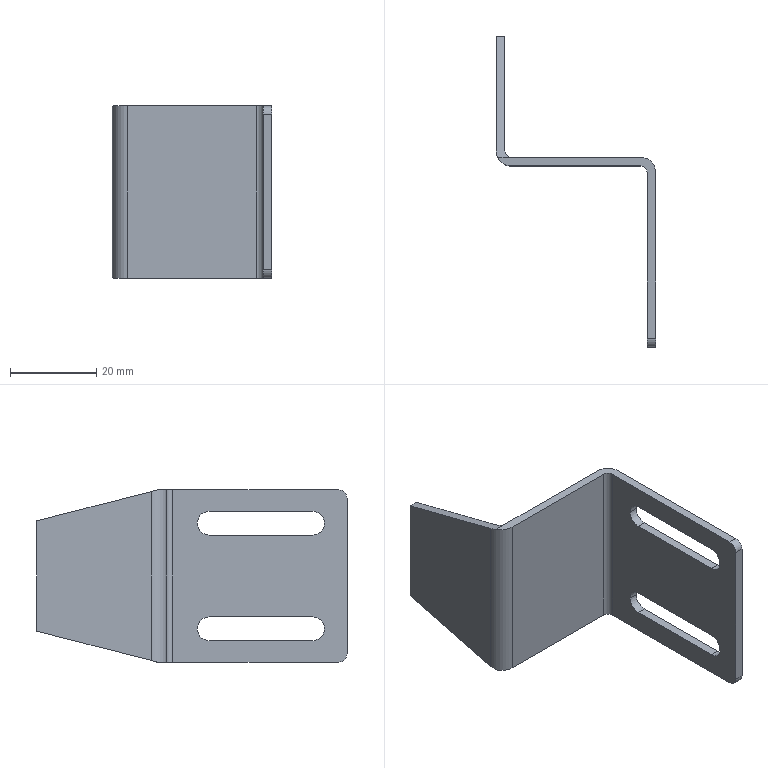Part | NX | features BREP 1 | 1 solid | 28 faces | box 37 x 72 x 40 mm | volume 7359 mm3 | plane 16 | cylinder 12 | commonest cylinder face diameters 5.5 x6 3 x2 4 x2 7 x2
STEP:
#1=CARTESIAN_POINT('',(0.,-7.25,-12.25));
#2=VERTEX_POINT('',#1);
#3=CARTESIAN_POINT('',(0.,-10.,-9.5));
#4=VERTEX_POINT('',#3);
#5=CARTESIAN_POINT('',(0.,-10.,-12.25));
#6=DIRECTION('',(1.,0.,0.));
#7=DIRECTION('',(0.,1.,0.));
#8=AXIS2_PLACEMENT_3D('',#5,#6,#7);
#9=CIRCLE('',#8,2.75);
#10=EDGE_CURVE('',#2,#4,#9,.T.);
#11=ORIENTED_EDGE('',*,*,#10,.F.);
#12=CARTESIAN_POINT('',(2.,-7.25,-12.25));
#13=VERTEX_POINT('',#12);
#14=CARTESIAN_POINT('',(-35.,-7.25,-12.25));
#15=DIRECTION('',(1.,0.,0.));
#16=VECTOR('',#15,1000.);
#17=LINE('',#14,#16);
#18=EDGE_CURVE('',#2,#13,#17,.T.);
#19=ORIENTED_EDGE('',*,*,#18,.T.);
#20=CARTESIAN_POINT('',(2.,-10.,-9.5));
#21=VERTEX_POINT('',#20);
#22=CARTESIAN_POINT('',(2.,-10.,-12.25));
#23=DIRECTION('',(1.,0.,0.));
#24=DIRECTION('',(0.,-1.,0.));
#25=AXIS2_PLACEMENT_3D('',#22,#23,#24);
#26=CIRCLE('',#25,2.75);
#27=EDGE_CURVE('',#13,#21,#26,.T.);
#28=ORIENTED_EDGE('',*,*,#27,.T.);
#29=CARTESIAN_POINT('',(-35.,-10.,-9.5));
#30=DIRECTION('',(1.,0.,0.));
#31=VECTOR('',#30,1000.);
#32=LINE('',#29,#31);
#33=EDGE_CURVE('',#4,#21,#32,.T.);
#34=ORIENTED_EDGE('',*,*,#33,.F.);
#35=EDGE_LOOP('',(#11,#19,#28,#34));
#36=FACE_BOUND('',#35,.T.);
#37=CARTESIAN_POINT('',(-35.,-10.,-12.25));
#38=DIRECTION('',(1.,0.,0.));
#39=DIRECTION('',(0.,1.,0.));
#40=AXIS2_PLACEMENT_3D('',#37,#38,#39);
#41=CYLINDRICAL_SURFACE('',#40,2.75);
#42=ADVANCED_FACE('',(#36),#41,.F.);
#43=CARTESIAN_POINT('',(0.,-7.25,12.25));
#44=VERTEX_POINT('',#43);
#45=CARTESIAN_POINT('',(0.,-10.,15.));
#46=VERTEX_POINT('',#45);
#47=CARTESIAN_POINT('',(0.,-10.,12.25));
#48=DIRECTION('',(1.,0.,0.));
#49=DIRECTION('',(0.,1.,0.));
#50=AXIS2_PLACEMENT_3D('',#47,#48,#49);
#51=CIRCLE('',#50,2.75);
#52=EDGE_CURVE('',#44,#46,#51,.T.);
#53=ORIENTED_EDGE('',*,*,#52,.F.);
#54=CARTESIAN_POINT('',(2.,-7.25,12.25));
#55=VERTEX_POINT('',#54);
#56=CARTESIAN_POINT('',(-35.,-7.25,12.25));
#57=DIRECTION('',(1.,0.,0.));
#58=VECTOR('',#57,1000.);
#59=LINE('',#56,#58);
#60=EDGE_CURVE('',#44,#55,#59,.T.);
#61=ORIENTED_EDGE('',*,*,#60,.T.);
#62=CARTESIAN_POINT('',(2.,-10.,15.));
#63=VERTEX_POINT('',#62);
#64=CARTESIAN_POINT('',(2.,-10.,12.25));
#65=DIRECTION('',(1.,0.,0.));
#66=DIRECTION('',(0.,1.,0.));
#67=AXIS2_PLACEMENT_3D('',#64,#65,#66);
#68=CIRCLE('',#67,2.75);
#69=EDGE_CURVE('',#55,#63,#68,.T.);
#70=ORIENTED_EDGE('',*,*,#69,.T.);
#71=CARTESIAN_POINT('',(-35.,-10.,15.));
#72=DIRECTION('',(1.,0.,0.));
#73=VECTOR('',#72,1000.);
#74=LINE('',#71,#73);
#75=EDGE_CURVE('',#46,#63,#74,.T.);
#76=ORIENTED_EDGE('',*,*,#75,.F.);
#77=EDGE_LOOP('',(#53,#61,#70,#76));
#78=FACE_BOUND('',#77,.T.);
#79=CARTESIAN_POINT('',(-35.,-10.,12.25));
#80=DIRECTION('',(1.,0.,0.));
#81=DIRECTION('',(0.,1.,0.));
#82=AXIS2_PLACEMENT_3D('',#79,#80,#81);
#83=CYLINDRICAL_SURFACE('',#82,2.75);
#84=ADVANCED_FACE('',(#78),#83,.F.);
#85=CARTESIAN_POINT('',(2.,-42.,18.));
#86=VERTEX_POINT('',#85);
#87=CARTESIAN_POINT('',(2.,-42.,-18.));
#88=VERTEX_POINT('',#87);
#89=CARTESIAN_POINT('',(2.,-42.,20.));
#90=DIRECTION('',(0.,0.,-1.));
#91=VECTOR('',#90,1000.);
#92=LINE('',#89,#91);
#93=EDGE_CURVE('',#86,#88,#92,.T.);
#94=ORIENTED_EDGE('',*,*,#93,.T.);
#95=CARTESIAN_POINT('',(2.,-40.,-20.));
#96=VERTEX_POINT('',#95);
#97=CARTESIAN_POINT('',(2.,-40.,-18.));
#98=DIRECTION('',(1.,0.,0.));
#99=DIRECTION('',(0.,-1.,0.));
#100=AXIS2_PLACEMENT_3D('',#97,#98,#99);
#101=CIRCLE('',#100,2.);
#102=EDGE_CURVE('',#88,#96,#101,.T.);
#103=ORIENTED_EDGE('',*,*,#102,.T.);
#104=CARTESIAN_POINT('',(2.,-1.5,-20.));
#105=VERTEX_POINT('',#104);
#106=CARTESIAN_POINT('',(2.,2.,-20.));
#107=DIRECTION('',(0.,1.,0.));
#108=VECTOR('',#107,1000.);
#109=LINE('',#106,#108);
#110=EDGE_CURVE('',#96,#105,#109,.T.);
#111=ORIENTED_EDGE('',*,*,#110,.T.);
#112=CARTESIAN_POINT('',(2.,-1.5,20.));
#113=VERTEX_POINT('',#112);
#114=CARTESIAN_POINT('',(2.,-1.5,20.));
#115=DIRECTION('',(0.,0.,1.));
#116=VECTOR('',#115,1000.);
#117=LINE('',#114,#116);
#118=EDGE_CURVE('',#105,#113,#117,.T.);
#119=ORIENTED_EDGE('',*,*,#118,.T.);
#120=CARTESIAN_POINT('',(2.,-40.,20.));
#121=VERTEX_POINT('',#120);
#122=CARTESIAN_POINT('',(2.,2.,20.));
#123=DIRECTION('',(0.,1.,0.));
#124=VECTOR('',#123,1000.);
#125=LINE('',#122,#124);
#126=EDGE_CURVE('',#121,#113,#125,.T.);
#127=ORIENTED_EDGE('',*,*,#126,.F.);
#128=CARTESIAN_POINT('',(2.,-40.,18.));
#129=DIRECTION('',(1.,0.,0.));
#130=DIRECTION('',(0.,-1.,0.));
#131=AXIS2_PLACEMENT_3D('',#128,#129,#130);
#132=CIRCLE('',#131,2.);
#133=EDGE_CURVE('',#121,#86,#132,.T.);
#134=ORIENTED_EDGE('',*,*,#133,.T.);
#135=EDGE_LOOP('',(#94,#103,#111,#119,#127,#134));
#136=FACE_BOUND('',#135,.T.);
#137=CARTESIAN_POINT('',(2.,-34.,-9.5));
#138=VERTEX_POINT('',#137);
#139=CARTESIAN_POINT('',(2.,-10.,-9.5));
#140=DIRECTION('',(0.,-1.,0.));
#141=VECTOR('',#140,1000.);
#142=LINE('',#139,#141);
#143=EDGE_CURVE('',#21,#138,#142,.T.);
#144=ORIENTED_EDGE('',*,*,#143,.F.);
#145=ORIENTED_EDGE('',*,*,#27,.F.);
#146=CARTESIAN_POINT('',(2.,-10.,-15.));
#147=VERTEX_POINT('',#146);
#148=CARTESIAN_POINT('',(2.,-10.,-12.25));
#149=DIRECTION('',(1.,0.,0.));
#150=DIRECTION('',(0.,-1.,0.));
#151=AXIS2_PLACEMENT_3D('',#148,#149,#150);
#152=CIRCLE('',#151,2.75);
#153=EDGE_CURVE('',#147,#13,#152,.T.);
#154=ORIENTED_EDGE('',*,*,#153,.F.);
#155=CARTESIAN_POINT('',(2.,-34.,-15.));
#156=VERTEX_POINT('',#155);
#157=CARTESIAN_POINT('',(2.,-10.,-15.));
#158=DIRECTION('',(0.,1.,0.));
#159=VECTOR('',#158,1000.);
#160=LINE('',#157,#159);
#161=EDGE_CURVE('',#156,#147,#160,.T.);
#162=ORIENTED_EDGE('',*,*,#161,.F.);
#163=CARTESIAN_POINT('',(2.,-34.,-12.25));
#164=DIRECTION('',(1.,0.,0.));
#165=DIRECTION('',(0.,-1.,0.));
#166=AXIS2_PLACEMENT_3D('',#163,#164,#165);
#167=CIRCLE('',#166,2.75);
#168=EDGE_CURVE('',#138,#156,#167,.T.);
#169=ORIENTED_EDGE('',*,*,#168,.F.);
#170=EDGE_LOOP('',(#144,#145,#154,#162,#169));
#171=FACE_BOUND('',#170,.T.);
#172=CARTESIAN_POINT('',(2.,-34.,15.));
#173=VERTEX_POINT('',#172);
#174=CARTESIAN_POINT('',(2.,-10.,15.));
#175=DIRECTION('',(0.,-1.,0.));
#176=VECTOR('',#175,1000.);
#177=LINE('',#174,#176);
#178=EDGE_CURVE('',#63,#173,#177,.T.);
#179=ORIENTED_EDGE('',*,*,#178,.F.);
#180=ORIENTED_EDGE('',*,*,#69,.F.);
#181=CARTESIAN_POINT('',(2.,-10.,9.5));
#182=VERTEX_POINT('',#181);
#183=CARTESIAN_POINT('',(2.,-10.,12.25));
#184=DIRECTION('',(1.,0.,0.));
#185=DIRECTION('',(0.,1.,0.));
#186=AXIS2_PLACEMENT_3D('',#183,#184,#185);
#187=CIRCLE('',#186,2.75);
#188=EDGE_CURVE('',#182,#55,#187,.T.);
#189=ORIENTED_EDGE('',*,*,#188,.F.);
#190=CARTESIAN_POINT('',(2.,-34.,9.5));
#191=VERTEX_POINT('',#190);
#192=CARTESIAN_POINT('',(2.,-10.,9.5));
#193=DIRECTION('',(0.,1.,0.));
#194=VECTOR('',#193,1000.);
#195=LINE('',#192,#194);
#196=EDGE_CURVE('',#191,#182,#195,.T.);
#197=ORIENTED_EDGE('',*,*,#196,.F.);
#198=CARTESIAN_POINT('',(2.,-34.,12.25));
#199=DIRECTION('',(1.,0.,0.));
#200=DIRECTION('',(0.,1.,0.));
#201=AXIS2_PLACEMENT_3D('',#198,#199,#200);
#202=CIRCLE('',#201,2.75);
#203=EDGE_CURVE('',#173,#191,#202,.T.);
#204=ORIENTED_EDGE('',*,*,#203,.F.);
#205=EDGE_LOOP('',(#179,#180,#189,#197,#204));
#206=FACE_BOUND('',#205,.T.);
#207=CARTESIAN_POINT('',(2.,2.,20.));
#208=DIRECTION('',(-1.,0.,0.));
#209=DIRECTION('',(0.,1.,0.));
#210=AXIS2_PLACEMENT_3D('',#207,#208,#209);
#211=PLANE('',#210);
#212=ADVANCED_FACE('',(#136,#171,#206),#211,.F.);
#213=CARTESIAN_POINT('',(-1.5,2.,20.));
#214=VERTEX_POINT('',#213);
#215=CARTESIAN_POINT('',(-31.5,2.,20.));
#216=VERTEX_POINT('',#215);
#217=CARTESIAN_POINT('',(-33.,2.,20.));
#218=DIRECTION('',(-1.,0.,0.));
#219=VECTOR('',#218,1000.);
#220=LINE('',#217,#219);
#221=EDGE_CURVE('',#214,#216,#220,.T.);
#222=ORIENTED_EDGE('',*,*,#221,.F.);
#223=CARTESIAN_POINT('',(-1.5,2.,-20.));
#224=VERTEX_POINT('',#223);
#225=CARTESIAN_POINT('',(-1.5,2.,20.));
#226=DIRECTION('',(0.,0.,-1.));
#227=VECTOR('',#226,1000.);
#228=LINE('',#225,#227);
#229=EDGE_CURVE('',#214,#224,#228,.T.);
#230=ORIENTED_EDGE('',*,*,#229,.T.);
#231=CARTESIAN_POINT('',(-31.5,2.,-20.));
#232=VERTEX_POINT('',#231);
#233=CARTESIAN_POINT('',(-33.,2.,-20.));
#234=DIRECTION('',(-1.,0.,0.));
#235=VECTOR('',#234,1000.);
#236=LINE('',#233,#235);
#237=EDGE_CURVE('',#224,#232,#236,.T.);
#238=ORIENTED_EDGE('',*,*,#237,.T.);
#239=CARTESIAN_POINT('',(-31.5,2.,20.));
#240=DIRECTION('',(0.,0.,1.));
#241=VECTOR('',#240,1000.);
#242=LINE('',#239,#241);
#243=EDGE_CURVE('',#232,#216,#242,.T.);
#244=ORIENTED_EDGE('',*,*,#243,.T.);
#245=EDGE_LOOP('',(#222,#230,#238,#244));
#246=FACE_BOUND('',#245,.T.);
#247=CARTESIAN_POINT('',(-33.,2.,20.));
#248=DIRECTION('',(0.,-1.,0.));
#249=DIRECTION('',(-1.,0.,0.));
#250=AXIS2_PLACEMENT_3D('',#247,#248,#249);
#251=PLANE('',#250);
#252=ADVANCED_FACE('',(#246),#251,.F.);
#253=CARTESIAN_POINT('',(-33.,30.,12.8));
#254=VERTEX_POINT('',#253);
#255=CARTESIAN_POINT('',(-33.,3.5,19.614));
#256=VERTEX_POINT('',#255);
#257=CARTESIAN_POINT('',(-33.,28.263,13.247));
#258=DIRECTION('',(0.,-0.9685,0.249));
#259=VECTOR('',#258,1000.);
#260=LINE('',#257,#259);
#261=EDGE_CURVE('',#254,#256,#260,.T.);
#262=ORIENTED_EDGE('',*,*,#261,.T.);
#263=CARTESIAN_POINT('',(-33.,3.5,-19.614));
#264=VERTEX_POINT('',#263);
#265=CARTESIAN_POINT('',(-33.,3.5,-20.));
#266=DIRECTION('',(0.,0.,-1.));
#267=VECTOR('',#266,1000.);
#268=LINE('',#265,#267);
#269=EDGE_CURVE('',#256,#264,#268,.T.);
#270=ORIENTED_EDGE('',*,*,#269,.T.);
#271=CARTESIAN_POINT('',(-33.,30.,-12.8));
#272=VERTEX_POINT('',#271);
#273=CARTESIAN_POINT('',(-33.,37.911,-10.766));
#274=DIRECTION('',(0.,0.9685,0.249));
#275=VECTOR('',#274,1000.);
#276=LINE('',#273,#275);
#277=EDGE_CURVE('',#264,#272,#276,.T.);
#278=ORIENTED_EDGE('',*,*,#277,.T.);
#279=CARTESIAN_POINT('',(-33.,30.,20.));
#280=DIRECTION('',(0.,0.,-1.));
#281=VECTOR('',#280,1000.);
#282=LINE('',#279,#281);
#283=EDGE_CURVE('',#254,#272,#282,.T.);
#284=ORIENTED_EDGE('',*,*,#283,.F.);
#285=EDGE_LOOP('',(#262,#270,#278,#284));
#286=FACE_BOUND('',#285,.T.);
#287=CARTESIAN_POINT('',(-33.,30.,20.));
#288=DIRECTION('',(-1.,0.,0.));
#289=DIRECTION('',(0.,0.,1.));
#290=AXIS2_PLACEMENT_3D('',#287,#288,#289);
#291=PLANE('',#290);
#292=ADVANCED_FACE('',(#286),#291,.F.);
#293=ORIENTED_EDGE('',*,*,#283,.T.);
#294=CARTESIAN_POINT('',(-35.,30.,-12.8));
#295=VERTEX_POINT('',#294);
#296=CARTESIAN_POINT('',(-35.,30.,-12.8));
#297=DIRECTION('',(1.,0.,0.));
#298=VECTOR('',#297,1000.);
#299=LINE('',#296,#298);
#300=EDGE_CURVE('',#295,#272,#299,.T.);
#301=ORIENTED_EDGE('',*,*,#300,.F.);
#302=CARTESIAN_POINT('',(-35.,30.,12.8));
#303=VERTEX_POINT('',#302);
#304=CARTESIAN_POINT('',(-35.,30.,20.));
#305=DIRECTION('',(0.,0.,-1.));
#306=VECTOR('',#305,1000.);
#307=LINE('',#304,#306);
#308=EDGE_CURVE('',#303,#295,#307,.T.);
#309=ORIENTED_EDGE('',*,*,#308,.F.);
#310=CARTESIAN_POINT('',(-35.,30.,12.8));
#311=DIRECTION('',(1.,0.,0.));
#312=VECTOR('',#311,1000.);
#313=LINE('',#310,#312);
#314=EDGE_CURVE('',#303,#254,#313,.T.);
#315=ORIENTED_EDGE('',*,*,#314,.T.);
#316=EDGE_LOOP('',(#293,#301,#309,#315));
#317=FACE_BOUND('',#316,.T.);
#318=CARTESIAN_POINT('',(-35.,30.,20.));
#319=DIRECTION('',(0.,-1.,0.));
#320=DIRECTION('',(0.,0.,-1.));
#321=AXIS2_PLACEMENT_3D('',#318,#319,#320);
#322=PLANE('',#321);
#323=ADVANCED_FACE('',(#317),#322,.F.);
#324=CARTESIAN_POINT('',(-35.,3.5,-19.614));
#325=VERTEX_POINT('',#324);
#326=CARTESIAN_POINT('',(-35.,30.,-12.8));
#327=DIRECTION('',(0.,-0.9685,-0.249));
#328=VECTOR('',#327,1000.);
#329=LINE('',#326,#328);
#330=EDGE_CURVE('',#295,#325,#329,.T.);
#331=ORIENTED_EDGE('',*,*,#330,.T.);
#332=CARTESIAN_POINT('',(-35.,3.5,19.614));
#333=VERTEX_POINT('',#332);
#334=CARTESIAN_POINT('',(-35.,3.5,20.));
#335=DIRECTION('',(0.,0.,1.));
#336=VECTOR('',#335,1000.);
#337=LINE('',#334,#336);
#338=EDGE_CURVE('',#325,#333,#337,.T.);
#339=ORIENTED_EDGE('',*,*,#338,.T.);
#340=CARTESIAN_POINT('',(-35.,30.,12.8));
#341=DIRECTION('',(0.,0.9685,-0.249));
#342=VECTOR('',#341,1000.);
#343=LINE('',#340,#342);
#344=EDGE_CURVE('',#333,#303,#343,.T.);
#345=ORIENTED_EDGE('',*,*,#344,.T.);
#346=ORIENTED_EDGE('',*,*,#308,.T.);
#347=EDGE_LOOP('',(#331,#339,#345,#346));
#348=FACE_BOUND('',#347,.T.);
#349=CARTESIAN_POINT('',(-35.,0.,20.));
#350=DIRECTION('',(1.,0.,0.));
#351=DIRECTION('',(0.,1.,0.));
#352=AXIS2_PLACEMENT_3D('',#349,#350,#351);
#353=PLANE('',#352);
#354=ADVANCED_FACE('',(#348),#353,.F.);
#355=CARTESIAN_POINT('',(-31.5,0.,20.));
#356=VERTEX_POINT('',#355);
#357=CARTESIAN_POINT('',(-1.5,0.,20.));
#358=VERTEX_POINT('',#357);
#359=CARTESIAN_POINT('',(0.,0.,20.));
#360=DIRECTION('',(1.,0.,0.));
#361=VECTOR('',#360,1000.);
#362=LINE('',#359,#361);
#363=EDGE_CURVE('',#356,#358,#362,.T.);
#364=ORIENTED_EDGE('',*,*,#363,.F.);
#365=CARTESIAN_POINT('',(-31.5,0.,-20.));
#366=VERTEX_POINT('',#365);
#367=CARTESIAN_POINT('',(-31.5,0.,20.));
#368=DIRECTION('',(0.,0.,-1.));
#369=VECTOR('',#368,1000.);
#370=LINE('',#367,#369);
#371=EDGE_CURVE('',#356,#366,#370,.T.);
#372=ORIENTED_EDGE('',*,*,#371,.T.);
#373=CARTESIAN_POINT('',(-1.5,0.,-20.));
#374=VERTEX_POINT('',#373);
#375=CARTESIAN_POINT('',(0.,0.,-20.));
#376=DIRECTION('',(1.,0.,0.));
#377=VECTOR('',#376,1000.);
#378=LINE('',#375,#377);
#379=EDGE_CURVE('',#366,#374,#378,.T.);
#380=ORIENTED_EDGE('',*,*,#379,.T.);
#381=CARTESIAN_POINT('',(-1.5,0.,20.));
#382=DIRECTION('',(0.,0.,1.));
#383=VECTOR('',#382,1000.);
#384=LINE('',#381,#383);
#385=EDGE_CURVE('',#374,#358,#384,.T.);
#386=ORIENTED_EDGE('',*,*,#385,.T.);
#387=EDGE_LOOP('',(#364,#372,#380,#386));
#388=FACE_BOUND('',#387,.T.);
#389=CARTESIAN_POINT('',(0.,0.,20.));
#390=DIRECTION('',(0.,1.,0.));
#391=DIRECTION('',(1.,0.,0.));
#392=AXIS2_PLACEMENT_3D('',#389,#390,#391);
#393=PLANE('',#392);
#394=ADVANCED_FACE('',(#388),#393,.F.);
#395=CARTESIAN_POINT('',(0.,-1.5,-20.));
#396=VERTEX_POINT('',#395);
#397=CARTESIAN_POINT('',(0.,-40.,-20.));
#398=VERTEX_POINT('',#397);
#399=CARTESIAN_POINT('',(0.,-42.,-20.));
#400=DIRECTION('',(0.,-1.,0.));
#401=VECTOR('',#400,1000.);
#402=LINE('',#399,#401);
#403=EDGE_CURVE('',#396,#398,#402,.T.);
#404=ORIENTED_EDGE('',*,*,#403,.T.);
#405=CARTESIAN_POINT('',(0.,-42.,-18.));
#406=VERTEX_POINT('',#405);
#407=CARTESIAN_POINT('',(0.,-40.,-18.));
#408=DIRECTION('',(-1.,0.,0.));
#409=DIRECTION('',(0.,1.,0.));
#410=AXIS2_PLACEMENT_3D('',#407,#408,#409);
#411=CIRCLE('',#410,2.);
#412=EDGE_CURVE('',#398,#406,#411,.T.);
#413=ORIENTED_EDGE('',*,*,#412,.T.);
#414=CARTESIAN_POINT('',(0.,-42.,18.));
#415=VERTEX_POINT('',#414);
#416=CARTESIAN_POINT('',(0.,-42.,20.));
#417=DIRECTION('',(0.,0.,-1.));
#418=VECTOR('',#417,1000.);
#419=LINE('',#416,#418);
#420=EDGE_CURVE('',#415,#406,#419,.T.);
#421=ORIENTED_EDGE('',*,*,#420,.F.);
#422=CARTESIAN_POINT('',(0.,-40.,20.));
#423=VERTEX_POINT('',#422);
#424=CARTESIAN_POINT('',(0.,-40.,18.));
#425=DIRECTION('',(-1.,0.,0.));
#426=DIRECTION('',(0.,1.,0.));
#427=AXIS2_PLACEMENT_3D('',#424,#425,#426);
#428=CIRCLE('',#427,2.);
#429=EDGE_CURVE('',#415,#423,#428,.T.);
#430=ORIENTED_EDGE('',*,*,#429,.T.);
#431=CARTESIAN_POINT('',(0.,-1.5,20.));
#432=VERTEX_POINT('',#431);
#433=CARTESIAN_POINT('',(0.,-42.,20.));
#434=DIRECTION('',(0.,-1.,0.));
#435=VECTOR('',#434,1000.);
#436=LINE('',#433,#435);
#437=EDGE_CURVE('',#432,#423,#436,.T.);
#438=ORIENTED_EDGE('',*,*,#437,.F.);
#439=CARTESIAN_POINT('',(0.,-1.5,-20.));
#440=DIRECTION('',(0.,0.,-1.));
#441=VECTOR('',#440,1000.);
#442=LINE('',#439,#441);
#443=EDGE_CURVE('',#432,#396,#442,.T.);
#444=ORIENTED_EDGE('',*,*,#443,.T.);
#445=EDGE_LOOP('',(#404,#413,#421,#430,#438,#444));
#446=FACE_BOUND('',#445,.T.);
#447=CARTESIAN_POINT('',(0.,-34.,-15.));
#448=VERTEX_POINT('',#447);
#449=CARTESIAN_POINT('',(0.,-10.,-15.));
#450=VERTEX_POINT('',#449);
#451=CARTESIAN_POINT('',(0.,-42.,-15.));
#452=DIRECTION('',(0.,1.,0.));
#453=VECTOR('',#452,1000.);
#454=LINE('',#451,#453);
#455=EDGE_CURVE('',#448,#450,#454,.T.);
#456=ORIENTED_EDGE('',*,*,#455,.T.);
#457=CARTESIAN_POINT('',(0.,-10.,-12.25));
#458=DIRECTION('',(1.,0.,0.));
#459=DIRECTION('',(0.,1.,0.));
#460=AXIS2_PLACEMENT_3D('',#457,#458,#459);
#461=CIRCLE('',#460,2.75);
#462=EDGE_CURVE('',#450,#2,#461,.T.);
#463=ORIENTED_EDGE('',*,*,#462,.T.);
#464=ORIENTED_EDGE('',*,*,#10,.T.);
#465=CARTESIAN_POINT('',(0.,-34.,-9.5));
#466=VERTEX_POINT('',#465);
#467=CARTESIAN_POINT('',(0.,-42.,-9.5));
#468=DIRECTION('',(0.,-1.,0.));
#469=VECTOR('',#468,1000.);
#470=LINE('',#467,#469);
#471=EDGE_CURVE('',#4,#466,#470,.T.);
#472=ORIENTED_EDGE('',*,*,#471,.T.);
#473=CARTESIAN_POINT('',(0.,-34.,-12.25));
#474=DIRECTION('',(1.,0.,0.));
#475=DIRECTION('',(0.,1.,0.));
#476=AXIS2_PLACEMENT_3D('',#473,#474,#475);
#477=CIRCLE('',#476,2.75);
#478=EDGE_CURVE('',#466,#448,#477,.T.);
#479=ORIENTED_EDGE('',*,*,#478,.T.);
#480=EDGE_LOOP('',(#456,#463,#464,#472,#479));
#481=FACE_BOUND('',#480,.T.);
#482=CARTESIAN_POINT('',(0.,-34.,9.5));
#483=VERTEX_POINT('',#482);
#484=CARTESIAN_POINT('',(0.,-10.,9.5));
#485=VERTEX_POINT('',#484);
#486=CARTESIAN_POINT('',(0.,-42.,9.5));
#487=DIRECTION('',(0.,1.,0.));
#488=VECTOR('',#487,1000.);
#489=LINE('',#486,#488);
#490=EDGE_CURVE('',#483,#485,#489,.T.);
#491=ORIENTED_EDGE('',*,*,#490,.T.);
#492=CARTESIAN_POINT('',(0.,-10.,12.25));
#493=DIRECTION('',(1.,0.,0.));
#494=DIRECTION('',(0.,1.,0.));
#495=AXIS2_PLACEMENT_3D('',#492,#493,#494);
#496=CIRCLE('',#495,2.75);
#497=EDGE_CURVE('',#485,#44,#496,.T.);
#498=ORIENTED_EDGE('',*,*,#497,.T.);
#499=ORIENTED_EDGE('',*,*,#52,.T.);
#500=CARTESIAN_POINT('',(0.,-34.,15.));
#501=VERTEX_POINT('',#500);
#502=CARTESIAN_POINT('',(0.,-42.,15.));
#503=DIRECTION('',(0.,-1.,0.));
#504=VECTOR('',#503,1000.);
#505=LINE('',#502,#504);
#506=EDGE_CURVE('',#46,#501,#505,.T.);
#507=ORIENTED_EDGE('',*,*,#506,.T.);
#508=CARTESIAN_POINT('',(0.,-34.,12.25));
#509=DIRECTION('',(1.,0.,0.));
#510=DIRECTION('',(0.,1.,0.));
#511=AXIS2_PLACEMENT_3D('',#508,#509,#510);
#512=CIRCLE('',#511,2.75);
#513=EDGE_CURVE('',#501,#483,#512,.T.);
#514=ORIENTED_EDGE('',*,*,#513,.T.);
#515=EDGE_LOOP('',(#491,#498,#499,#507,#514));
#516=FACE_BOUND('',#515,.T.);
#517=CARTESIAN_POINT('',(0.,-42.,20.));
#518=DIRECTION('',(1.,0.,0.));
#519=DIRECTION('',(0.,1.,0.));
#520=AXIS2_PLACEMENT_3D('',#517,#518,#519);
#521=PLANE('',#520);
#522=ADVANCED_FACE('',(#446,#481,#516),#521,.F.);
#523=ORIENTED_EDGE('',*,*,#420,.T.);
#524=CARTESIAN_POINT('',(2.,-42.,-18.));
#525=DIRECTION('',(1.,0.,0.));
#526=VECTOR('',#525,1000.);
#527=LINE('',#524,#526);
#528=EDGE_CURVE('',#406,#88,#527,.T.);
#529=ORIENTED_EDGE('',*,*,#528,.T.);
#530=ORIENTED_EDGE('',*,*,#93,.F.);
#531=CARTESIAN_POINT('',(2.,-42.,18.));
#532=DIRECTION('',(-1.,0.,0.));
#533=VECTOR('',#532,1000.);
#534=LINE('',#531,#533);
#535=EDGE_CURVE('',#86,#415,#534,.T.);
#536=ORIENTED_EDGE('',*,*,#535,.T.);
#537=EDGE_LOOP('',(#523,#529,#530,#536));
#538=FACE_BOUND('',#537,.T.);
#539=CARTESIAN_POINT('',(2.,-42.,20.));
#540=DIRECTION('',(0.,1.,0.));
#541=DIRECTION('',(1.,0.,0.));
#542=AXIS2_PLACEMENT_3D('',#539,#540,#541);
#543=PLANE('',#542);
#544=ADVANCED_FACE('',(#538),#543,.F.);
#545=ORIENTED_EDGE('',*,*,#437,.T.);
#546=CARTESIAN_POINT('',(0.,-40.,20.));
#547=DIRECTION('',(1.,0.,0.));
#548=VECTOR('',#547,1000.);
#549=LINE('',#546,#548);
#550=EDGE_CURVE('',#423,#121,#549,.T.);
#551=ORIENTED_EDGE('',*,*,#550,.T.);
#552=ORIENTED_EDGE('',*,*,#126,.T.);
#553=CARTESIAN_POINT('',(-1.5,-1.5,20.));
#554=DIRECTION('',(0.,0.,1.));
#555=DIRECTION('',(-1.,0.,0.));
#556=AXIS2_PLACEMENT_3D('',#553,#554,#555);
#557=CIRCLE('',#556,3.5);
#558=EDGE_CURVE('',#113,#214,#557,.T.);
#559=ORIENTED_EDGE('',*,*,#558,.T.);
#560=ORIENTED_EDGE('',*,*,#221,.T.);
#561=CARTESIAN_POINT('',(-34.662,2.,20.));
#562=VERTEX_POINT('',#561);
#563=CARTESIAN_POINT('',(-35.,2.,20.));
#564=DIRECTION('',(1.,0.,0.));
#565=VECTOR('',#564,1000.);
#566=LINE('',#563,#565);
#567=EDGE_CURVE('',#562,#216,#566,.T.);
#568=ORIENTED_EDGE('',*,*,#567,.F.);
#569=CARTESIAN_POINT('',(-31.5,3.5,20.));
#570=DIRECTION('',(0.,0.,1.));
#571=DIRECTION('',(-1.,0.,0.));
#572=AXIS2_PLACEMENT_3D('',#569,#570,#571);
#573=CIRCLE('',#572,3.5);
#574=EDGE_CURVE('',#562,#356,#573,.T.);
#575=ORIENTED_EDGE('',*,*,#574,.T.);
#576=ORIENTED_EDGE('',*,*,#363,.T.);
#577=CARTESIAN_POINT('',(-1.5,-1.5,20.));
#578=DIRECTION('',(0.,0.,-1.));
#579=DIRECTION('',(-1.,0.,0.));
#580=AXIS2_PLACEMENT_3D('',#577,#578,#579);
#581=CIRCLE('',#580,1.5);
#582=EDGE_CURVE('',#358,#432,#581,.T.);
#583=ORIENTED_EDGE('',*,*,#582,.T.);
#584=EDGE_LOOP('',(#545,#551,#552,#559,#560,#568,#575,#576,#583));
#585=FACE_BOUND('',#584,.T.);
#586=CARTESIAN_POINT('',(0.,0.,20.));
#587=DIRECTION('',(0.,0.,-1.));
#588=DIRECTION('',(0.,-1.,0.));
#589=AXIS2_PLACEMENT_3D('',#586,#587,#588);
#590=PLANE('',#589);
#591=ADVANCED_FACE('',(#585),#590,.F.);
#592=ORIENTED_EDGE('',*,*,#110,.F.);
#593=CARTESIAN_POINT('',(0.,-40.,-20.));
#594=DIRECTION('',(-1.,0.,0.));
#595=VECTOR('',#594,1000.);
#596=LINE('',#593,#595);
#597=EDGE_CURVE('',#96,#398,#596,.T.);
#598=ORIENTED_EDGE('',*,*,#597,.T.);
#599=ORIENTED_EDGE('',*,*,#403,.F.);
#600=CARTESIAN_POINT('',(-1.5,-1.5,-20.));
#601=DIRECTION('',(0.,0.,1.));
#602=DIRECTION('',(-1.,0.,0.));
#603=AXIS2_PLACEMENT_3D('',#600,#601,#602);
#604=CIRCLE('',#603,1.5);
#605=EDGE_CURVE('',#396,#374,#604,.T.);
#606=ORIENTED_EDGE('',*,*,#605,.T.);
#607=ORIENTED_EDGE('',*,*,#379,.F.);
#608=CARTESIAN_POINT('',(-34.662,2.,-20.));
#609=VERTEX_POINT('',#608);
#610=CARTESIAN_POINT('',(-31.5,3.5,-20.));
#611=DIRECTION('',(0.,0.,-1.));
#612=DIRECTION('',(-1.,0.,0.));
#613=AXIS2_PLACEMENT_3D('',#610,#611,#612);
#614=CIRCLE('',#613,3.5);
#615=EDGE_CURVE('',#366,#609,#614,.T.);
#616=ORIENTED_EDGE('',*,*,#615,.T.);
#617=CARTESIAN_POINT('',(-35.,2.,-20.));
#618=DIRECTION('',(1.,0.,0.));
#619=VECTOR('',#618,1000.);
#620=LINE('',#617,#619);
#621=EDGE_CURVE('',#609,#232,#620,.T.);
#622=ORIENTED_EDGE('',*,*,#621,.T.);
#623=ORIENTED_EDGE('',*,*,#237,.F.);
#624=CARTESIAN_POINT('',(-1.5,-1.5,-20.));
#625=DIRECTION('',(0.,0.,-1.));
#626=DIRECTION('',(-1.,0.,0.));
#627=AXIS2_PLACEMENT_3D('',#624,#625,#626);
#628=CIRCLE('',#627,3.5);
#629=EDGE_CURVE('',#224,#105,#628,.T.);
#630=ORIENTED_EDGE('',*,*,#629,.T.);
#631=EDGE_LOOP('',(#592,#598,#599,#606,#607,#616,#622,#623,#630));
#632=FACE_BOUND('',#631,.T.);
#633=CARTESIAN_POINT('',(0.,0.,-20.));
#634=DIRECTION('',(0.,0.,-1.));
#635=DIRECTION('',(0.,-1.,0.));
#636=AXIS2_PLACEMENT_3D('',#633,#634,#635);
#637=PLANE('',#636);
#638=ADVANCED_FACE('',(#632),#637,.T.);
#639=ORIENTED_EDGE('',*,*,#344,.F.);
#640=CARTESIAN_POINT('',(-35.,3.5,19.614));
#641=CARTESIAN_POINT('',(-35.,2.979,19.748));
#642=CARTESIAN_POINT('',(-34.886,2.471,19.879));
#643=CARTESIAN_POINT('',(-34.662,2.,20.));
#644=(BOUNDED_CURVE()B_SPLINE_CURVE(3,(#640,#641,#642,#643),.UNSPECIFIED.,.F.,.F.)B_SPLINE_CURVE_WITH_KNOTS((4,4),(1.571,2.014),.UNSPECIFIED.)CURVE()GEOMETRIC_REPRESENTATION_ITEM()RATIONAL_B_SPLINE_CURVE((1.,0.9837,0.9837,1.))REPRESENTATION_ITEM(''));
#645=EDGE_CURVE('',#333,#562,#644,.T.);
#646=ORIENTED_EDGE('',*,*,#645,.T.);
#647=ORIENTED_EDGE('',*,*,#567,.T.);
#648=CARTESIAN_POINT('',(-31.5,2.,20.));
#649=CARTESIAN_POINT('',(-32.379,2.,20.));
#650=CARTESIAN_POINT('',(-33.,2.621,19.84));
#651=CARTESIAN_POINT('',(-33.,3.5,19.614));
#652=(BOUNDED_CURVE()B_SPLINE_CURVE(3,(#648,#649,#650,#651),.UNSPECIFIED.,.F.,.F.)B_SPLINE_CURVE_WITH_KNOTS((4,4),(0.,1.571),.UNSPECIFIED.)CURVE()GEOMETRIC_REPRESENTATION_ITEM()RATIONAL_B_SPLINE_CURVE((1.,0.8047,0.8047,1.))REPRESENTATION_ITEM(''));
#653=EDGE_CURVE('',#216,#256,#652,.T.);
#654=ORIENTED_EDGE('',*,*,#653,.T.);
#655=ORIENTED_EDGE('',*,*,#261,.F.);
#656=ORIENTED_EDGE('',*,*,#314,.F.);
#657=EDGE_LOOP('',(#639,#646,#647,#654,#655,#656));
#658=FACE_BOUND('',#657,.T.);
#659=CARTESIAN_POINT('',(-35.,30.,12.8));
#660=DIRECTION('',(0.,-0.249,-0.9685));
#661=DIRECTION('',(0.,-0.9685,0.249));
#662=AXIS2_PLACEMENT_3D('',#659,#660,#661);
#663=PLANE('',#662);
#664=ADVANCED_FACE('',(#658),#663,.F.);
#665=ORIENTED_EDGE('',*,*,#621,.F.);
#666=CARTESIAN_POINT('',(-34.662,2.,-20.));
#667=CARTESIAN_POINT('',(-34.886,2.471,-19.879));
#668=CARTESIAN_POINT('',(-35.,2.979,-19.748));
#669=CARTESIAN_POINT('',(-35.,3.5,-19.614));
#670=(BOUNDED_CURVE()B_SPLINE_CURVE(3,(#666,#667,#668,#669),.UNSPECIFIED.,.F.,.F.)B_SPLINE_CURVE_WITH_KNOTS((4,4),(1.128,1.571),.UNSPECIFIED.)CURVE()GEOMETRIC_REPRESENTATION_ITEM()RATIONAL_B_SPLINE_CURVE((1.,0.9837,0.9837,1.))REPRESENTATION_ITEM(''));
#671=EDGE_CURVE('',#609,#325,#670,.T.);
#672=ORIENTED_EDGE('',*,*,#671,.T.);
#673=ORIENTED_EDGE('',*,*,#330,.F.);
#674=ORIENTED_EDGE('',*,*,#300,.T.);
#675=ORIENTED_EDGE('',*,*,#277,.F.);
#676=CARTESIAN_POINT('',(-33.,3.5,-19.614));
#677=CARTESIAN_POINT('',(-33.,2.621,-19.84));
#678=CARTESIAN_POINT('',(-32.379,2.,-20.));
#679=CARTESIAN_POINT('',(-31.5,2.,-20.));
#680=(BOUNDED_CURVE()B_SPLINE_CURVE(3,(#676,#677,#678,#679),.UNSPECIFIED.,.F.,.F.)B_SPLINE_CURVE_WITH_KNOTS((4,4),(1.571,3.142),.UNSPECIFIED.)CURVE()GEOMETRIC_REPRESENTATION_ITEM()RATIONAL_B_SPLINE_CURVE((1.,0.8047,0.8047,1.))REPRESENTATION_ITEM(''));
#681=EDGE_CURVE('',#264,#232,#680,.T.);
#682=ORIENTED_EDGE('',*,*,#681,.T.);
#683=EDGE_LOOP('',(#665,#672,#673,#674,#675,#682));
#684=FACE_BOUND('',#683,.T.);
#685=CARTESIAN_POINT('',(-35.,30.,-12.8));
#686=DIRECTION('',(0.,-0.249,0.9685));
#687=DIRECTION('',(-1.,0.,0.));
#688=AXIS2_PLACEMENT_3D('',#685,#686,#687);
#689=PLANE('',#688);
#690=ADVANCED_FACE('',(#684),#689,.F.);
#691=ORIENTED_EDGE('',*,*,#60,.F.);
#692=ORIENTED_EDGE('',*,*,#497,.F.);
#693=CARTESIAN_POINT('',(-35.,-10.,9.5));
#694=DIRECTION('',(1.,0.,0.));
#695=VECTOR('',#694,1000.);
#696=LINE('',#693,#695);
#697=EDGE_CURVE('',#485,#182,#696,.T.);
#698=ORIENTED_EDGE('',*,*,#697,.T.);
#699=ORIENTED_EDGE('',*,*,#188,.T.);
#700=EDGE_LOOP('',(#691,#692,#698,#699));
#701=FACE_BOUND('',#700,.T.);
#702=CARTESIAN_POINT('',(-35.,-10.,12.25));
#703=DIRECTION('',(1.,0.,0.));
#704=DIRECTION('',(0.,1.,0.));
#705=AXIS2_PLACEMENT_3D('',#702,#703,#704);
#706=CYLINDRICAL_SURFACE('',#705,2.75);
#707=ADVANCED_FACE('',(#701),#706,.F.);
#708=CARTESIAN_POINT('',(-35.,-34.,9.5));
#709=DIRECTION('',(1.,0.,0.));
#710=VECTOR('',#709,1000.);
#711=LINE('',#708,#710);
#712=EDGE_CURVE('',#483,#191,#711,.T.);
#713=ORIENTED_EDGE('',*,*,#712,.T.);
#714=ORIENTED_EDGE('',*,*,#196,.T.);
#715=ORIENTED_EDGE('',*,*,#697,.F.);
#716=ORIENTED_EDGE('',*,*,#490,.F.);
#717=EDGE_LOOP('',(#713,#714,#715,#716));
#718=FACE_BOUND('',#717,.T.);
#719=CARTESIAN_POINT('',(-35.,-10.,9.5));
#720=DIRECTION('',(0.,0.,-1.));
#721=DIRECTION('',(-1.,0.,0.));
#722=AXIS2_PLACEMENT_3D('',#719,#720,#721);
#723=PLANE('',#722);
#724=ADVANCED_FACE('',(#718),#723,.F.);
#725=CARTESIAN_POINT('',(-35.,-34.,15.));
#726=DIRECTION('',(1.,0.,0.));
#727=VECTOR('',#726,1000.);
#728=LINE('',#725,#727);
#729=EDGE_CURVE('',#501,#173,#728,.T.);
#730=ORIENTED_EDGE('',*,*,#729,.T.);
#731=ORIENTED_EDGE('',*,*,#203,.T.);
#732=ORIENTED_EDGE('',*,*,#712,.F.);
#733=ORIENTED_EDGE('',*,*,#513,.F.);
#734=EDGE_LOOP('',(#730,#731,#732,#733));
#735=FACE_BOUND('',#734,.T.);
#736=CARTESIAN_POINT('',(-35.,-34.,12.25));
#737=DIRECTION('',(1.,0.,0.));
#738=DIRECTION('',(0.,1.,0.));
#739=AXIS2_PLACEMENT_3D('',#736,#737,#738);
#740=CYLINDRICAL_SURFACE('',#739,2.75);
#741=ADVANCED_FACE('',(#735),#740,.F.);
#742=ORIENTED_EDGE('',*,*,#75,.T.);
#743=ORIENTED_EDGE('',*,*,#178,.T.);
#744=ORIENTED_EDGE('',*,*,#729,.F.);
#745=ORIENTED_EDGE('',*,*,#506,.F.);
#746=EDGE_LOOP('',(#742,#743,#744,#745));
#747=FACE_BOUND('',#746,.T.);
#748=CARTESIAN_POINT('',(-35.,-10.,15.));
#749=DIRECTION('',(0.,0.,1.));
#750=DIRECTION('',(0.,-1.,0.));
#751=AXIS2_PLACEMENT_3D('',#748,#749,#750);
#752=PLANE('',#751);
#753=ADVANCED_FACE('',(#747),#752,.F.);
#754=ORIENTED_EDGE('',*,*,#18,.F.);
#755=ORIENTED_EDGE('',*,*,#462,.F.);
#756=CARTESIAN_POINT('',(-35.,-10.,-15.));
#757=DIRECTION('',(1.,0.,0.));
#758=VECTOR('',#757,1000.);
#759=LINE('',#756,#758);
#760=EDGE_CURVE('',#450,#147,#759,.T.);
#761=ORIENTED_EDGE('',*,*,#760,.T.);
#762=ORIENTED_EDGE('',*,*,#153,.T.);
#763=EDGE_LOOP('',(#754,#755,#761,#762));
#764=FACE_BOUND('',#763,.T.);
#765=CARTESIAN_POINT('',(-35.,-10.,-12.25));
#766=DIRECTION('',(1.,0.,0.));
#767=DIRECTION('',(0.,1.,0.));
#768=AXIS2_PLACEMENT_3D('',#765,#766,#767);
#769=CYLINDRICAL_SURFACE('',#768,2.75);
#770=ADVANCED_FACE('',(#764),#769,.F.);
#771=CARTESIAN_POINT('',(-35.,-34.,-15.));
#772=DIRECTION('',(1.,0.,0.));
#773=VECTOR('',#772,1000.);
#774=LINE('',#771,#773);
#775=EDGE_CURVE('',#448,#156,#774,.T.);
#776=ORIENTED_EDGE('',*,*,#775,.T.);
#777=ORIENTED_EDGE('',*,*,#161,.T.);
#778=ORIENTED_EDGE('',*,*,#760,.F.);
#779=ORIENTED_EDGE('',*,*,#455,.F.);
#780=EDGE_LOOP('',(#776,#777,#778,#779));
#781=FACE_BOUND('',#780,.T.);
#782=CARTESIAN_POINT('',(-35.,-10.,-15.));
#783=DIRECTION('',(0.,0.,-1.));
#784=DIRECTION('',(-1.,0.,0.));
#785=AXIS2_PLACEMENT_3D('',#782,#783,#784);
#786=PLANE('',#785);
#787=ADVANCED_FACE('',(#781),#786,.F.);
#788=CARTESIAN_POINT('',(-35.,-34.,-9.5));
#789=DIRECTION('',(1.,0.,0.));
#790=VECTOR('',#789,1000.);
#791=LINE('',#788,#790);
#792=EDGE_CURVE('',#466,#138,#791,.T.);
#793=ORIENTED_EDGE('',*,*,#792,.T.);
#794=ORIENTED_EDGE('',*,*,#168,.T.);
#795=ORIENTED_EDGE('',*,*,#775,.F.);
#796=ORIENTED_EDGE('',*,*,#478,.F.);
#797=EDGE_LOOP('',(#793,#794,#795,#796));
#798=FACE_BOUND('',#797,.T.);
#799=CARTESIAN_POINT('',(-35.,-34.,-12.25));
#800=DIRECTION('',(1.,0.,0.));
#801=DIRECTION('',(0.,1.,0.));
#802=AXIS2_PLACEMENT_3D('',#799,#800,#801);
#803=CYLINDRICAL_SURFACE('',#802,2.75);
#804=ADVANCED_FACE('',(#798),#803,.F.);
#805=ORIENTED_EDGE('',*,*,#33,.T.);
#806=ORIENTED_EDGE('',*,*,#143,.T.);
#807=ORIENTED_EDGE('',*,*,#792,.F.);
#808=ORIENTED_EDGE('',*,*,#471,.F.);
#809=EDGE_LOOP('',(#805,#806,#807,#808));
#810=FACE_BOUND('',#809,.T.);
#811=CARTESIAN_POINT('',(-35.,-10.,-9.5));
#812=DIRECTION('',(0.,0.,1.));
#813=DIRECTION('',(0.,-1.,0.));
#814=AXIS2_PLACEMENT_3D('',#811,#812,#813);
#815=PLANE('',#814);
#816=ADVANCED_FACE('',(#810),#815,.F.);
#817=ORIENTED_EDGE('',*,*,#412,.F.);
#818=ORIENTED_EDGE('',*,*,#597,.F.);
#819=ORIENTED_EDGE('',*,*,#102,.F.);
#820=ORIENTED_EDGE('',*,*,#528,.F.);
#821=EDGE_LOOP('',(#817,#818,#819,#820));
#822=FACE_BOUND('',#821,.T.);
#823=CARTESIAN_POINT('',(2.,-40.,-18.));
#824=DIRECTION('',(-1.,0.,0.));
#825=DIRECTION('',(0.,0.,1.));
#826=AXIS2_PLACEMENT_3D('',#823,#824,#825);
#827=CYLINDRICAL_SURFACE('',#826,2.);
#828=ADVANCED_FACE('',(#822),#827,.T.);
#829=ORIENTED_EDGE('',*,*,#429,.F.);
#830=ORIENTED_EDGE('',*,*,#535,.F.);
#831=ORIENTED_EDGE('',*,*,#133,.F.);
#832=ORIENTED_EDGE('',*,*,#550,.F.);
#833=EDGE_LOOP('',(#829,#830,#831,#832));
#834=FACE_BOUND('',#833,.T.);
#835=CARTESIAN_POINT('',(0.,-40.,18.));
#836=DIRECTION('',(1.,0.,0.));
#837=DIRECTION('',(0.,0.,-1.));
#838=AXIS2_PLACEMENT_3D('',#835,#836,#837);
#839=CYLINDRICAL_SURFACE('',#838,2.);
#840=ADVANCED_FACE('',(#834),#839,.T.);
#841=ORIENTED_EDGE('',*,*,#645,.F.);
#842=ORIENTED_EDGE('',*,*,#338,.F.);
#843=ORIENTED_EDGE('',*,*,#671,.F.);
#844=ORIENTED_EDGE('',*,*,#615,.F.);
#845=ORIENTED_EDGE('',*,*,#371,.F.);
#846=ORIENTED_EDGE('',*,*,#574,.F.);
#847=EDGE_LOOP('',(#841,#842,#843,#844,#845,#846));
#848=FACE_BOUND('',#847,.T.);
#849=CARTESIAN_POINT('',(-31.5,3.5,20.));
#850=DIRECTION('',(0.,0.,-1.));
#851=DIRECTION('',(-1.,0.,0.));
#852=AXIS2_PLACEMENT_3D('',#849,#850,#851);
#853=CYLINDRICAL_SURFACE('',#852,3.5);
#854=ADVANCED_FACE('',(#848),#853,.T.);
#855=ORIENTED_EDGE('',*,*,#558,.F.);
#856=ORIENTED_EDGE('',*,*,#118,.F.);
#857=ORIENTED_EDGE('',*,*,#629,.F.);
#858=ORIENTED_EDGE('',*,*,#229,.F.);
#859=EDGE_LOOP('',(#855,#856,#857,#858));
#860=FACE_BOUND('',#859,.T.);
#861=CARTESIAN_POINT('',(-1.5,-1.5,20.));
#862=DIRECTION('',(0.,0.,-1.));
#863=DIRECTION('',(-1.,0.,0.));
#864=AXIS2_PLACEMENT_3D('',#861,#862,#863);
#865=CYLINDRICAL_SURFACE('',#864,3.5);
#866=ADVANCED_FACE('',(#860),#865,.T.);
#867=ORIENTED_EDGE('',*,*,#653,.F.);
#868=ORIENTED_EDGE('',*,*,#243,.F.);
#869=ORIENTED_EDGE('',*,*,#681,.F.);
#870=ORIENTED_EDGE('',*,*,#269,.F.);
#871=EDGE_LOOP('',(#867,#868,#869,#870));
#872=FACE_BOUND('',#871,.T.);
#873=CARTESIAN_POINT('',(-31.5,3.5,20.));
#874=DIRECTION('',(0.,0.,1.));
#875=DIRECTION('',(1.,0.,0.));
#876=AXIS2_PLACEMENT_3D('',#873,#874,#875);
#877=CYLINDRICAL_SURFACE('',#876,1.5);
#878=ADVANCED_FACE('',(#872),#877,.F.);
#879=ORIENTED_EDGE('',*,*,#582,.F.);
#880=ORIENTED_EDGE('',*,*,#385,.F.);
#881=ORIENTED_EDGE('',*,*,#605,.F.);
#882=ORIENTED_EDGE('',*,*,#443,.F.);
#883=EDGE_LOOP('',(#879,#880,#881,#882));
#884=FACE_BOUND('',#883,.T.);
#885=CARTESIAN_POINT('',(-1.5,-1.5,20.));
#886=DIRECTION('',(0.,0.,1.));
#887=DIRECTION('',(1.,0.,0.));
#888=AXIS2_PLACEMENT_3D('',#885,#886,#887);
#889=CYLINDRICAL_SURFACE('',#888,1.5);
#890=ADVANCED_FACE('',(#884),#889,.F.);
#891=CLOSED_SHELL('',(#42,#84,#212,#252,#292,#323,#354,#394,#522,#544,#591,#638,#664,#690,#707,#724,#741,#753,#770,#787,#804,#816,#828,#840,#854,#866,#878,#890));
#892=MANIFOLD_SOLID_BREP('',#891);
#893=(LENGTH_UNIT()NAMED_UNIT(*)SI_UNIT(.MILLI.,.METRE.));
#894=UNCERTAINTY_MEASURE_WITH_UNIT(LENGTH_MEASURE(0.00001),#893,'','');
#895=(NAMED_UNIT(*)PLANE_ANGLE_UNIT()SI_UNIT($,.RADIAN.));
#896=(NAMED_UNIT(*)SI_UNIT($,.STERADIAN.)SOLID_ANGLE_UNIT());
#897=(GEOMETRIC_REPRESENTATION_CONTEXT(3)GLOBAL_UNCERTAINTY_ASSIGNED_CONTEXT((#894))GLOBAL_UNIT_ASSIGNED_CONTEXT((#893,#895,#896))REPRESENTATION_CONTEXT('',''));
#898=ADVANCED_BREP_SHAPE_REPRESENTATION('',(#892),#897);